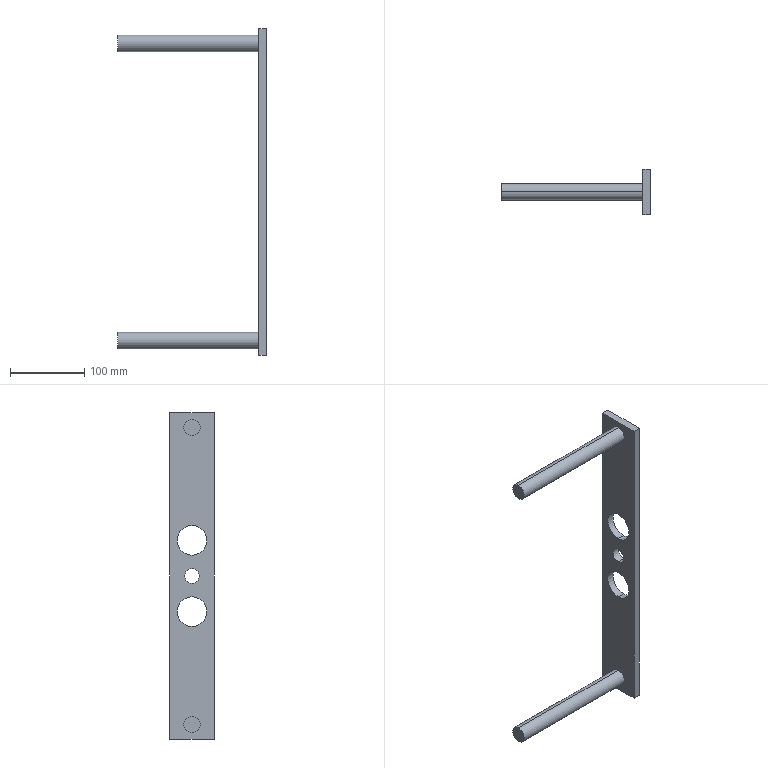Part | STEP file | 1 solid | 18 faces | box 200 x 60 x 440 mm | volume 380176 mm3 | cylinder 10 | plane 8 | commonest cylinder face diameters 22 x4 40 x4 20 x2
STEP:
#1=CARTESIAN_POINT('',(0.,0.,0.));
#2=DIRECTION('',(0.,0.,1.));
#3=DIRECTION('',(1.,0.,0.));
#4=AXIS2_PLACEMENT_3D('',#1,#2,#3);
#5=CARTESIAN_POINT('',(-10.,30.,-10.));
#6=VERTEX_POINT('',#5);
#7=CARTESIAN_POINT('',(0.,30.,-10.));
#8=VERTEX_POINT('',#7);
#9=CARTESIAN_POINT('',(13.,30.,-10.));
#10=DIRECTION('',(1.,0.,0.));
#11=VECTOR('',#10,1.);
#12=LINE('',#9,#11);
#13=CARTESIAN_POINT('',(13.,30.,0.));
#14=DIRECTION('',(1.,0.,0.));
#15=DIRECTION('',(0.,0.,-1.));
#16=AXIS2_PLACEMENT_3D('',#13,#14,#15);
#17=CYLINDRICAL_SURFACE('',#16,10.);
#18=CARTESIAN_POINT('',(6.283,0.));
#19=DIRECTION('',(0.,1.));
#20=VECTOR('',#19,1.);
#21=LINE('',#18,#20);
#22=(GEOMETRIC_REPRESENTATION_CONTEXT(2)PARAMETRIC_REPRESENTATION_CONTEXT()REPRESENTATION_CONTEXT('',''));
#23=DEFINITIONAL_REPRESENTATION('',(#21),#22);
#24=PCURVE('',#17,#23);
#25=CARTESIAN_POINT('',(13.,30.,0.));
#26=DIRECTION('',(1.,0.,0.));
#27=DIRECTION('',(0.,0.,-1.));
#28=AXIS2_PLACEMENT_3D('',#25,#26,#27);
#29=CYLINDRICAL_SURFACE('',#28,10.);
#30=CARTESIAN_POINT('',(0.,0.));
#31=DIRECTION('',(0.,1.));
#32=VECTOR('',#31,1.);
#33=LINE('',#30,#32);
#34=(GEOMETRIC_REPRESENTATION_CONTEXT(2)PARAMETRIC_REPRESENTATION_CONTEXT()REPRESENTATION_CONTEXT('',''));
#35=DEFINITIONAL_REPRESENTATION('',(#33),#34);
#36=PCURVE('',#29,#35);
#37=SURFACE_CURVE('',#12,(#24,#36),.PCURVE_S1.);
#38=EDGE_CURVE('',#6,#8,#37,.T.);
#39=ORIENTED_EDGE('',*,*,#38,.T.);
#40=CARTESIAN_POINT('',(0.,30.,10.));
#41=VERTEX_POINT('',#40);
#42=CARTESIAN_POINT('',(0.,30.,0.));
#43=DIRECTION('',(-1.,0.,0.));
#44=DIRECTION('',(0.,0.,-1.));
#45=AXIS2_PLACEMENT_3D('',#42,#43,#44);
#46=CIRCLE('',#45,10.);
#47=CARTESIAN_POINT('',(6.283,-13.));
#48=DIRECTION('',(-1.,0.));
#49=VECTOR('',#48,1.);
#50=LINE('',#47,#49);
#51=(GEOMETRIC_REPRESENTATION_CONTEXT(2)PARAMETRIC_REPRESENTATION_CONTEXT()REPRESENTATION_CONTEXT('',''));
#52=DEFINITIONAL_REPRESENTATION('',(#50),#51);
#53=PCURVE('',#17,#52);
#54=CARTESIAN_POINT('',(0.,60.,220.));
#55=DIRECTION('',(1.,0.,0.));
#56=DIRECTION('',(0.,1.,0.));
#57=AXIS2_PLACEMENT_3D('',#54,#55,#56);
#58=PLANE('',#57);
#59=CARTESIAN_POINT('',(-30.,-230.));
#60=CARTESIAN_POINT('',(-47.321,-230.));
#61=CARTESIAN_POINT('',(-38.66,-215.));
#62=CARTESIAN_POINT('',(-30.,-200.));
#63=CARTESIAN_POINT('',(-21.34,-215.));
#64=CARTESIAN_POINT('',(-12.679,-230.));
#65=CARTESIAN_POINT('',(-30.,-230.));
#66=(BOUNDED_CURVE()B_SPLINE_CURVE(2,(#59,#60,#61,#62,#63,#64,#65),.UNSPECIFIED.,.T.,.F.)B_SPLINE_CURVE_WITH_KNOTS((1,2,2,2,2,1),(-2.094,0.,2.094,4.189,6.283,8.378),.UNSPECIFIED.)CURVE()GEOMETRIC_REPRESENTATION_ITEM()RATIONAL_B_SPLINE_CURVE((1.,0.5,1.,0.5,1.,0.5,1.))REPRESENTATION_ITEM(''));
#67=(GEOMETRIC_REPRESENTATION_CONTEXT(2)PARAMETRIC_REPRESENTATION_CONTEXT()REPRESENTATION_CONTEXT('',''));
#68=DEFINITIONAL_REPRESENTATION('',(#66),#67);
#69=PCURVE('',#58,#68);
#70=SURFACE_CURVE('',#46,(#53,#69),.PCURVE_S1.);
#71=EDGE_CURVE('',#8,#41,#70,.T.);
#72=ORIENTED_EDGE('',*,*,#71,.T.);
#73=CARTESIAN_POINT('',(-10.,30.,10.));
#74=VERTEX_POINT('',#73);
#75=CARTESIAN_POINT('',(13.,30.,10.));
#76=DIRECTION('',(1.,0.,0.));
#77=VECTOR('',#76,1.);
#78=LINE('',#75,#77);
#79=CARTESIAN_POINT('',(3.142,0.));
#80=DIRECTION('',(0.,1.));
#81=VECTOR('',#80,1.);
#82=LINE('',#79,#81);
#83=(GEOMETRIC_REPRESENTATION_CONTEXT(2)PARAMETRIC_REPRESENTATION_CONTEXT()REPRESENTATION_CONTEXT('',''));
#84=DEFINITIONAL_REPRESENTATION('',(#82),#83);
#85=PCURVE('',#17,#84);
#86=CARTESIAN_POINT('',(3.142,0.));
#87=DIRECTION('',(0.,1.));
#88=VECTOR('',#87,1.);
#89=LINE('',#86,#88);
#90=(GEOMETRIC_REPRESENTATION_CONTEXT(2)PARAMETRIC_REPRESENTATION_CONTEXT()REPRESENTATION_CONTEXT('',''));
#91=DEFINITIONAL_REPRESENTATION('',(#89),#90);
#92=PCURVE('',#29,#91);
#93=SURFACE_CURVE('',#78,(#85,#92),.PCURVE_S1.);
#94=EDGE_CURVE('',#74,#41,#93,.T.);
#95=ORIENTED_EDGE('',*,*,#94,.F.);
#96=CARTESIAN_POINT('',(-10.,30.,0.));
#97=DIRECTION('',(1.,0.,0.));
#98=DIRECTION('',(0.,0.,-1.));
#99=AXIS2_PLACEMENT_3D('',#96,#97,#98);
#100=CIRCLE('',#99,10.);
#101=CARTESIAN_POINT('',(0.,-23.));
#102=DIRECTION('',(1.,0.));
#103=VECTOR('',#102,1.);
#104=LINE('',#101,#103);
#105=(GEOMETRIC_REPRESENTATION_CONTEXT(2)PARAMETRIC_REPRESENTATION_CONTEXT()REPRESENTATION_CONTEXT('',''));
#106=DEFINITIONAL_REPRESENTATION('',(#104),#105);
#107=PCURVE('',#17,#106);
#108=CARTESIAN_POINT('',(-10.,60.,220.));
#109=DIRECTION('',(1.,0.,0.));
#110=DIRECTION('',(0.,1.,0.));
#111=AXIS2_PLACEMENT_3D('',#108,#109,#110);
#112=PLANE('',#111);
#113=CARTESIAN_POINT('',(-30.,-220.));
#114=DIRECTION('',(0.,-1.));
#115=AXIS2_PLACEMENT_2D('',#113,#114);
#116=CIRCLE('',#115,10.);
#117=(GEOMETRIC_REPRESENTATION_CONTEXT(2)PARAMETRIC_REPRESENTATION_CONTEXT()REPRESENTATION_CONTEXT('',''));
#118=DEFINITIONAL_REPRESENTATION('',(#116),#117);
#119=PCURVE('',#112,#118);
#120=SURFACE_CURVE('',#100,(#107,#119),.PCURVE_S1.);
#121=EDGE_CURVE('',#74,#6,#120,.T.);
#122=ORIENTED_EDGE('',*,*,#121,.T.);
#123=EDGE_LOOP('',(#39,#72,#95,#122));
#124=FACE_BOUND('',#123,.F.);
#125=ADVANCED_FACE('',(#124),#17,.F.);
#126=CARTESIAN_POINT('',(-10.,30.,28.));
#127=VERTEX_POINT('',#126);
#128=CARTESIAN_POINT('',(0.,30.,28.));
#129=VERTEX_POINT('',#128);
#130=CARTESIAN_POINT('',(13.,30.,28.));
#131=DIRECTION('',(1.,0.,0.));
#132=VECTOR('',#131,1.);
#133=LINE('',#130,#132);
#134=CARTESIAN_POINT('',(13.,30.,48.));
#135=DIRECTION('',(1.,0.,0.));
#136=DIRECTION('',(0.,0.,-1.));
#137=AXIS2_PLACEMENT_3D('',#134,#135,#136);
#138=CYLINDRICAL_SURFACE('',#137,20.);
#139=CARTESIAN_POINT('',(6.283,0.));
#140=DIRECTION('',(0.,1.));
#141=VECTOR('',#140,1.);
#142=LINE('',#139,#141);
#143=(GEOMETRIC_REPRESENTATION_CONTEXT(2)PARAMETRIC_REPRESENTATION_CONTEXT()REPRESENTATION_CONTEXT('',''));
#144=DEFINITIONAL_REPRESENTATION('',(#142),#143);
#145=PCURVE('',#138,#144);
#146=CARTESIAN_POINT('',(13.,30.,48.));
#147=DIRECTION('',(1.,0.,0.));
#148=DIRECTION('',(0.,0.,-1.));
#149=AXIS2_PLACEMENT_3D('',#146,#147,#148);
#150=CYLINDRICAL_SURFACE('',#149,20.);
#151=CARTESIAN_POINT('',(0.,0.));
#152=DIRECTION('',(0.,1.));
#153=VECTOR('',#152,1.);
#154=LINE('',#151,#153);
#155=(GEOMETRIC_REPRESENTATION_CONTEXT(2)PARAMETRIC_REPRESENTATION_CONTEXT()REPRESENTATION_CONTEXT('',''));
#156=DEFINITIONAL_REPRESENTATION('',(#154),#155);
#157=PCURVE('',#150,#156);
#158=SURFACE_CURVE('',#133,(#145,#157),.PCURVE_S1.);
#159=EDGE_CURVE('',#127,#129,#158,.T.);
#160=ORIENTED_EDGE('',*,*,#159,.T.);
#161=CARTESIAN_POINT('',(0.,30.,68.));
#162=VERTEX_POINT('',#161);
#163=CARTESIAN_POINT('',(0.,30.,48.));
#164=DIRECTION('',(-1.,0.,0.));
#165=DIRECTION('',(0.,0.,-1.));
#166=AXIS2_PLACEMENT_3D('',#163,#164,#165);
#167=CIRCLE('',#166,20.);
#168=CARTESIAN_POINT('',(6.283,-13.));
#169=DIRECTION('',(-1.,0.));
#170=VECTOR('',#169,1.);
#171=LINE('',#168,#170);
#172=(GEOMETRIC_REPRESENTATION_CONTEXT(2)PARAMETRIC_REPRESENTATION_CONTEXT()REPRESENTATION_CONTEXT('',''));
#173=DEFINITIONAL_REPRESENTATION('',(#171),#172);
#174=PCURVE('',#138,#173);
#175=CARTESIAN_POINT('',(-30.,-192.));
#176=CARTESIAN_POINT('',(-64.641,-192.));
#177=CARTESIAN_POINT('',(-47.321,-162.));
#178=CARTESIAN_POINT('',(-30.,-132.));
#179=CARTESIAN_POINT('',(-12.679,-162.));
#180=CARTESIAN_POINT('',(4.641,-192.));
#181=CARTESIAN_POINT('',(-30.,-192.));
#182=(BOUNDED_CURVE()B_SPLINE_CURVE(2,(#175,#176,#177,#178,#179,#180,#181),.UNSPECIFIED.,.T.,.F.)B_SPLINE_CURVE_WITH_KNOTS((1,2,2,2,2,1),(-2.094,0.,2.094,4.189,6.283,8.378),.UNSPECIFIED.)CURVE()GEOMETRIC_REPRESENTATION_ITEM()RATIONAL_B_SPLINE_CURVE((1.,0.5,1.,0.5,1.,0.5,1.))REPRESENTATION_ITEM(''));
#183=(GEOMETRIC_REPRESENTATION_CONTEXT(2)PARAMETRIC_REPRESENTATION_CONTEXT()REPRESENTATION_CONTEXT('',''));
#184=DEFINITIONAL_REPRESENTATION('',(#182),#183);
#185=PCURVE('',#58,#184);
#186=SURFACE_CURVE('',#167,(#174,#185),.PCURVE_S1.);
#187=EDGE_CURVE('',#129,#162,#186,.T.);
#188=ORIENTED_EDGE('',*,*,#187,.T.);
#189=CARTESIAN_POINT('',(-10.,30.,68.));
#190=VERTEX_POINT('',#189);
#191=CARTESIAN_POINT('',(13.,30.,68.));
#192=DIRECTION('',(1.,0.,0.));
#193=VECTOR('',#192,1.);
#194=LINE('',#191,#193);
#195=CARTESIAN_POINT('',(3.142,0.));
#196=DIRECTION('',(0.,1.));
#197=VECTOR('',#196,1.);
#198=LINE('',#195,#197);
#199=(GEOMETRIC_REPRESENTATION_CONTEXT(2)PARAMETRIC_REPRESENTATION_CONTEXT()REPRESENTATION_CONTEXT('',''));
#200=DEFINITIONAL_REPRESENTATION('',(#198),#199);
#201=PCURVE('',#138,#200);
#202=CARTESIAN_POINT('',(3.142,0.));
#203=DIRECTION('',(0.,1.));
#204=VECTOR('',#203,1.);
#205=LINE('',#202,#204);
#206=(GEOMETRIC_REPRESENTATION_CONTEXT(2)PARAMETRIC_REPRESENTATION_CONTEXT()REPRESENTATION_CONTEXT('',''));
#207=DEFINITIONAL_REPRESENTATION('',(#205),#206);
#208=PCURVE('',#150,#207);
#209=SURFACE_CURVE('',#194,(#201,#208),.PCURVE_S1.);
#210=EDGE_CURVE('',#190,#162,#209,.T.);
#211=ORIENTED_EDGE('',*,*,#210,.F.);
#212=CARTESIAN_POINT('',(-10.,30.,48.));
#213=DIRECTION('',(1.,0.,0.));
#214=DIRECTION('',(0.,0.,-1.));
#215=AXIS2_PLACEMENT_3D('',#212,#213,#214);
#216=CIRCLE('',#215,20.);
#217=CARTESIAN_POINT('',(0.,-23.));
#218=DIRECTION('',(1.,0.));
#219=VECTOR('',#218,1.);
#220=LINE('',#217,#219);
#221=(GEOMETRIC_REPRESENTATION_CONTEXT(2)PARAMETRIC_REPRESENTATION_CONTEXT()REPRESENTATION_CONTEXT('',''));
#222=DEFINITIONAL_REPRESENTATION('',(#220),#221);
#223=PCURVE('',#138,#222);
#224=CARTESIAN_POINT('',(-30.,-172.));
#225=DIRECTION('',(0.,-1.));
#226=AXIS2_PLACEMENT_2D('',#224,#225);
#227=CIRCLE('',#226,20.);
#228=(GEOMETRIC_REPRESENTATION_CONTEXT(2)PARAMETRIC_REPRESENTATION_CONTEXT()REPRESENTATION_CONTEXT('',''));
#229=DEFINITIONAL_REPRESENTATION('',(#227),#228);
#230=PCURVE('',#112,#229);
#231=SURFACE_CURVE('',#216,(#223,#230),.PCURVE_S1.);
#232=EDGE_CURVE('',#190,#127,#231,.T.);
#233=ORIENTED_EDGE('',*,*,#232,.T.);
#234=EDGE_LOOP('',(#160,#188,#211,#233));
#235=FACE_BOUND('',#234,.F.);
#236=ADVANCED_FACE('',(#235),#138,.F.);
#237=CARTESIAN_POINT('',(-10.,30.,-68.));
#238=VERTEX_POINT('',#237);
#239=CARTESIAN_POINT('',(0.,30.,-68.));
#240=VERTEX_POINT('',#239);
#241=CARTESIAN_POINT('',(13.,30.,-68.));
#242=DIRECTION('',(1.,0.,0.));
#243=VECTOR('',#242,1.);
#244=LINE('',#241,#243);
#245=CARTESIAN_POINT('',(13.,30.,-48.));
#246=DIRECTION('',(1.,0.,0.));
#247=DIRECTION('',(0.,0.,-1.));
#248=AXIS2_PLACEMENT_3D('',#245,#246,#247);
#249=CYLINDRICAL_SURFACE('',#248,20.);
#250=CARTESIAN_POINT('',(6.283,0.));
#251=DIRECTION('',(0.,1.));
#252=VECTOR('',#251,1.);
#253=LINE('',#250,#252);
#254=(GEOMETRIC_REPRESENTATION_CONTEXT(2)PARAMETRIC_REPRESENTATION_CONTEXT()REPRESENTATION_CONTEXT('',''));
#255=DEFINITIONAL_REPRESENTATION('',(#253),#254);
#256=PCURVE('',#249,#255);
#257=CARTESIAN_POINT('',(13.,30.,-48.));
#258=DIRECTION('',(1.,0.,0.));
#259=DIRECTION('',(0.,0.,-1.));
#260=AXIS2_PLACEMENT_3D('',#257,#258,#259);
#261=CYLINDRICAL_SURFACE('',#260,20.);
#262=CARTESIAN_POINT('',(0.,0.));
#263=DIRECTION('',(0.,1.));
#264=VECTOR('',#263,1.);
#265=LINE('',#262,#264);
#266=(GEOMETRIC_REPRESENTATION_CONTEXT(2)PARAMETRIC_REPRESENTATION_CONTEXT()REPRESENTATION_CONTEXT('',''));
#267=DEFINITIONAL_REPRESENTATION('',(#265),#266);
#268=PCURVE('',#261,#267);
#269=SURFACE_CURVE('',#244,(#256,#268),.PCURVE_S1.);
#270=EDGE_CURVE('',#238,#240,#269,.T.);
#271=ORIENTED_EDGE('',*,*,#270,.T.);
#272=CARTESIAN_POINT('',(0.,30.,-28.));
#273=VERTEX_POINT('',#272);
#274=CARTESIAN_POINT('',(0.,30.,-48.));
#275=DIRECTION('',(-1.,0.,0.));
#276=DIRECTION('',(0.,0.,-1.));
#277=AXIS2_PLACEMENT_3D('',#274,#275,#276);
#278=CIRCLE('',#277,20.);
#279=CARTESIAN_POINT('',(6.283,-13.));
#280=DIRECTION('',(-1.,0.));
#281=VECTOR('',#280,1.);
#282=LINE('',#279,#281);
#283=(GEOMETRIC_REPRESENTATION_CONTEXT(2)PARAMETRIC_REPRESENTATION_CONTEXT()REPRESENTATION_CONTEXT('',''));
#284=DEFINITIONAL_REPRESENTATION('',(#282),#283);
#285=PCURVE('',#249,#284);
#286=CARTESIAN_POINT('',(-30.,-288.));
#287=CARTESIAN_POINT('',(-64.641,-288.));
#288=CARTESIAN_POINT('',(-47.321,-258.));
#289=CARTESIAN_POINT('',(-30.,-228.));
#290=CARTESIAN_POINT('',(-12.679,-258.));
#291=CARTESIAN_POINT('',(4.641,-288.));
#292=CARTESIAN_POINT('',(-30.,-288.));
#293=(BOUNDED_CURVE()B_SPLINE_CURVE(2,(#286,#287,#288,#289,#290,#291,#292),.UNSPECIFIED.,.T.,.F.)B_SPLINE_CURVE_WITH_KNOTS((1,2,2,2,2,1),(-2.094,0.,2.094,4.189,6.283,8.378),.UNSPECIFIED.)CURVE()GEOMETRIC_REPRESENTATION_ITEM()RATIONAL_B_SPLINE_CURVE((1.,0.5,1.,0.5,1.,0.5,1.))REPRESENTATION_ITEM(''));
#294=(GEOMETRIC_REPRESENTATION_CONTEXT(2)PARAMETRIC_REPRESENTATION_CONTEXT()REPRESENTATION_CONTEXT('',''));
#295=DEFINITIONAL_REPRESENTATION('',(#293),#294);
#296=PCURVE('',#58,#295);
#297=SURFACE_CURVE('',#278,(#285,#296),.PCURVE_S1.);
#298=EDGE_CURVE('',#240,#273,#297,.T.);
#299=ORIENTED_EDGE('',*,*,#298,.T.);
#300=CARTESIAN_POINT('',(-10.,30.,-28.));
#301=VERTEX_POINT('',#300);
#302=CARTESIAN_POINT('',(13.,30.,-28.));
#303=DIRECTION('',(1.,0.,0.));
#304=VECTOR('',#303,1.);
#305=LINE('',#302,#304);
#306=CARTESIAN_POINT('',(3.142,0.));
#307=DIRECTION('',(0.,1.));
#308=VECTOR('',#307,1.);
#309=LINE('',#306,#308);
#310=(GEOMETRIC_REPRESENTATION_CONTEXT(2)PARAMETRIC_REPRESENTATION_CONTEXT()REPRESENTATION_CONTEXT('',''));
#311=DEFINITIONAL_REPRESENTATION('',(#309),#310);
#312=PCURVE('',#249,#311);
#313=CARTESIAN_POINT('',(3.142,0.));
#314=DIRECTION('',(0.,1.));
#315=VECTOR('',#314,1.);
#316=LINE('',#313,#315);
#317=(GEOMETRIC_REPRESENTATION_CONTEXT(2)PARAMETRIC_REPRESENTATION_CONTEXT()REPRESENTATION_CONTEXT('',''));
#318=DEFINITIONAL_REPRESENTATION('',(#316),#317);
#319=PCURVE('',#261,#318);
#320=SURFACE_CURVE('',#305,(#312,#319),.PCURVE_S1.);
#321=EDGE_CURVE('',#301,#273,#320,.T.);
#322=ORIENTED_EDGE('',*,*,#321,.F.);
#323=CARTESIAN_POINT('',(-10.,30.,-48.));
#324=DIRECTION('',(1.,0.,0.));
#325=DIRECTION('',(0.,0.,-1.));
#326=AXIS2_PLACEMENT_3D('',#323,#324,#325);
#327=CIRCLE('',#326,20.);
#328=CARTESIAN_POINT('',(0.,-23.));
#329=DIRECTION('',(1.,0.));
#330=VECTOR('',#329,1.);
#331=LINE('',#328,#330);
#332=(GEOMETRIC_REPRESENTATION_CONTEXT(2)PARAMETRIC_REPRESENTATION_CONTEXT()REPRESENTATION_CONTEXT('',''));
#333=DEFINITIONAL_REPRESENTATION('',(#331),#332);
#334=PCURVE('',#249,#333);
#335=CARTESIAN_POINT('',(-30.,-268.));
#336=DIRECTION('',(0.,-1.));
#337=AXIS2_PLACEMENT_2D('',#335,#336);
#338=CIRCLE('',#337,20.);
#339=(GEOMETRIC_REPRESENTATION_CONTEXT(2)PARAMETRIC_REPRESENTATION_CONTEXT()REPRESENTATION_CONTEXT('',''));
#340=DEFINITIONAL_REPRESENTATION('',(#338),#339);
#341=PCURVE('',#112,#340);
#342=SURFACE_CURVE('',#327,(#334,#341),.PCURVE_S1.);
#343=EDGE_CURVE('',#301,#238,#342,.T.);
#344=ORIENTED_EDGE('',*,*,#343,.T.);
#345=EDGE_LOOP('',(#271,#299,#322,#344));
#346=FACE_BOUND('',#345,.F.);
#347=ADVANCED_FACE('',(#346),#249,.F.);
#348=CARTESIAN_POINT('',(-10.,30.,211.));
#349=VERTEX_POINT('',#348);
#350=CARTESIAN_POINT('',(-10.,30.,189.));
#351=VERTEX_POINT('',#350);
#352=CARTESIAN_POINT('',(-10.,30.,200.));
#353=DIRECTION('',(-1.,0.,0.));
#354=DIRECTION('',(0.,0.,1.));
#355=AXIS2_PLACEMENT_3D('',#352,#353,#354);
#356=CIRCLE('',#355,11.);
#357=CARTESIAN_POINT('',(-200.,30.,200.));
#358=DIRECTION('',(-1.,0.,0.));
#359=DIRECTION('',(0.,0.,1.));
#360=AXIS2_PLACEMENT_3D('',#357,#358,#359);
#361=CYLINDRICAL_SURFACE('',#360,11.);
#362=CARTESIAN_POINT('',(0.,-190.));
#363=DIRECTION('',(1.,0.));
#364=VECTOR('',#363,1.);
#365=LINE('',#362,#364);
#366=(GEOMETRIC_REPRESENTATION_CONTEXT(2)PARAMETRIC_REPRESENTATION_CONTEXT()REPRESENTATION_CONTEXT('',''));
#367=DEFINITIONAL_REPRESENTATION('',(#365),#366);
#368=PCURVE('',#361,#367);
#369=CARTESIAN_POINT('',(-30.,-9.));
#370=CARTESIAN_POINT('',(-10.947,-9.));
#371=CARTESIAN_POINT('',(-20.474,-25.5));
#372=CARTESIAN_POINT('',(-30.,-42.));
#373=CARTESIAN_POINT('',(-39.526,-25.5));
#374=CARTESIAN_POINT('',(-49.053,-9.));
#375=CARTESIAN_POINT('',(-30.,-9.));
#376=(BOUNDED_CURVE()B_SPLINE_CURVE(2,(#369,#370,#371,#372,#373,#374,#375),.UNSPECIFIED.,.T.,.F.)B_SPLINE_CURVE_WITH_KNOTS((1,2,2,2,2,1),(-2.094,0.,2.094,4.189,6.283,8.378),.UNSPECIFIED.)CURVE()GEOMETRIC_REPRESENTATION_ITEM()RATIONAL_B_SPLINE_CURVE((1.,0.5,1.,0.5,1.,0.5,1.))REPRESENTATION_ITEM(''));
#377=(GEOMETRIC_REPRESENTATION_CONTEXT(2)PARAMETRIC_REPRESENTATION_CONTEXT()REPRESENTATION_CONTEXT('',''));
#378=DEFINITIONAL_REPRESENTATION('',(#376),#377);
#379=PCURVE('',#112,#378);
#380=SURFACE_CURVE('',#356,(#368,#379),.PCURVE_S1.);
#381=EDGE_CURVE('',#349,#351,#380,.T.);
#382=ORIENTED_EDGE('',*,*,#381,.T.);
#383=CARTESIAN_POINT('',(-200.,30.,189.));
#384=VERTEX_POINT('',#383);
#385=CARTESIAN_POINT('',(-200.,30.,189.));
#386=DIRECTION('',(-1.,0.,0.));
#387=VECTOR('',#386,1.);
#388=LINE('',#385,#387);
#389=CARTESIAN_POINT('',(3.142,0.));
#390=DIRECTION('',(0.,1.));
#391=VECTOR('',#390,1.);
#392=LINE('',#389,#391);
#393=(GEOMETRIC_REPRESENTATION_CONTEXT(2)PARAMETRIC_REPRESENTATION_CONTEXT()REPRESENTATION_CONTEXT('',''));
#394=DEFINITIONAL_REPRESENTATION('',(#392),#393);
#395=PCURVE('',#361,#394);
#396=CARTESIAN_POINT('',(-200.,30.,200.));
#397=DIRECTION('',(-1.,0.,0.));
#398=DIRECTION('',(0.,0.,1.));
#399=AXIS2_PLACEMENT_3D('',#396,#397,#398);
#400=CYLINDRICAL_SURFACE('',#399,11.);
#401=CARTESIAN_POINT('',(3.142,0.));
#402=DIRECTION('',(0.,1.));
#403=VECTOR('',#402,1.);
#404=LINE('',#401,#403);
#405=(GEOMETRIC_REPRESENTATION_CONTEXT(2)PARAMETRIC_REPRESENTATION_CONTEXT()REPRESENTATION_CONTEXT('',''));
#406=DEFINITIONAL_REPRESENTATION('',(#404),#405);
#407=PCURVE('',#400,#406);
#408=SURFACE_CURVE('',#388,(#395,#407),.PCURVE_S1.);
#409=EDGE_CURVE('',#351,#384,#408,.T.);
#410=ORIENTED_EDGE('',*,*,#409,.T.);
#411=CARTESIAN_POINT('',(-200.,30.,211.));
#412=VERTEX_POINT('',#411);
#413=CARTESIAN_POINT('',(-200.,30.,200.));
#414=DIRECTION('',(1.,0.,0.));
#415=DIRECTION('',(0.,0.,1.));
#416=AXIS2_PLACEMENT_3D('',#413,#414,#415);
#417=CIRCLE('',#416,11.);
#418=CARTESIAN_POINT('',(6.283,0.));
#419=DIRECTION('',(-1.,0.));
#420=VECTOR('',#419,1.);
#421=LINE('',#418,#420);
#422=(GEOMETRIC_REPRESENTATION_CONTEXT(2)PARAMETRIC_REPRESENTATION_CONTEXT()REPRESENTATION_CONTEXT('',''));
#423=DEFINITIONAL_REPRESENTATION('',(#421),#422);
#424=PCURVE('',#361,#423);
#425=CARTESIAN_POINT('',(-200.,30.,200.));
#426=DIRECTION('',(1.,0.,0.));
#427=DIRECTION('',(0.,1.,0.));
#428=AXIS2_PLACEMENT_3D('',#425,#426,#427);
#429=PLANE('',#428);
#430=CARTESIAN_POINT('',(0.,0.));
#431=DIRECTION('',(0.,1.));
#432=AXIS2_PLACEMENT_2D('',#430,#431);
#433=CIRCLE('',#432,11.);
#434=(GEOMETRIC_REPRESENTATION_CONTEXT(2)PARAMETRIC_REPRESENTATION_CONTEXT()REPRESENTATION_CONTEXT('',''));
#435=DEFINITIONAL_REPRESENTATION('',(#433),#434);
#436=PCURVE('',#429,#435);
#437=SURFACE_CURVE('',#417,(#424,#436),.PCURVE_S1.);
#438=EDGE_CURVE('',#384,#412,#437,.T.);
#439=ORIENTED_EDGE('',*,*,#438,.T.);
#440=CARTESIAN_POINT('',(-200.,30.,211.));
#441=DIRECTION('',(-1.,0.,0.));
#442=VECTOR('',#441,1.);
#443=LINE('',#440,#442);
#444=CARTESIAN_POINT('',(0.,0.));
#445=DIRECTION('',(0.,1.));
#446=VECTOR('',#445,1.);
#447=LINE('',#444,#446);
#448=(GEOMETRIC_REPRESENTATION_CONTEXT(2)PARAMETRIC_REPRESENTATION_CONTEXT()REPRESENTATION_CONTEXT('',''));
#449=DEFINITIONAL_REPRESENTATION('',(#447),#448);
#450=PCURVE('',#361,#449);
#451=CARTESIAN_POINT('',(6.283,0.));
#452=DIRECTION('',(0.,1.));
#453=VECTOR('',#452,1.);
#454=LINE('',#451,#453);
#455=(GEOMETRIC_REPRESENTATION_CONTEXT(2)PARAMETRIC_REPRESENTATION_CONTEXT()REPRESENTATION_CONTEXT('',''));
#456=DEFINITIONAL_REPRESENTATION('',(#454),#455);
#457=PCURVE('',#400,#456);
#458=SURFACE_CURVE('',#443,(#450,#457),.PCURVE_S1.);
#459=EDGE_CURVE('',#349,#412,#458,.T.);
#460=ORIENTED_EDGE('',*,*,#459,.F.);
#461=EDGE_LOOP('',(#382,#410,#439,#460));
#462=FACE_BOUND('',#461,.T.);
#463=ADVANCED_FACE('',(#462),#361,.T.);
#464=CARTESIAN_POINT('',(-10.,30.,-189.));
#465=VERTEX_POINT('',#464);
#466=CARTESIAN_POINT('',(-10.,30.,-211.));
#467=VERTEX_POINT('',#466);
#468=CARTESIAN_POINT('',(-10.,30.,-200.));
#469=DIRECTION('',(-1.,0.,0.));
#470=DIRECTION('',(0.,0.,1.));
#471=AXIS2_PLACEMENT_3D('',#468,#469,#470);
#472=CIRCLE('',#471,11.);
#473=CARTESIAN_POINT('',(-200.,30.,-200.));
#474=DIRECTION('',(-1.,0.,0.));
#475=DIRECTION('',(0.,0.,1.));
#476=AXIS2_PLACEMENT_3D('',#473,#474,#475);
#477=CYLINDRICAL_SURFACE('',#476,11.);
#478=CARTESIAN_POINT('',(0.,-190.));
#479=DIRECTION('',(1.,0.));
#480=VECTOR('',#479,1.);
#481=LINE('',#478,#480);
#482=(GEOMETRIC_REPRESENTATION_CONTEXT(2)PARAMETRIC_REPRESENTATION_CONTEXT()REPRESENTATION_CONTEXT('',''));
#483=DEFINITIONAL_REPRESENTATION('',(#481),#482);
#484=PCURVE('',#477,#483);
#485=CARTESIAN_POINT('',(-30.,-409.));
#486=CARTESIAN_POINT('',(-10.947,-409.));
#487=CARTESIAN_POINT('',(-20.474,-425.5));
#488=CARTESIAN_POINT('',(-30.,-442.));
#489=CARTESIAN_POINT('',(-39.526,-425.5));
#490=CARTESIAN_POINT('',(-49.053,-409.));
#491=CARTESIAN_POINT('',(-30.,-409.));
#492=(BOUNDED_CURVE()B_SPLINE_CURVE(2,(#485,#486,#487,#488,#489,#490,#491),.UNSPECIFIED.,.T.,.F.)B_SPLINE_CURVE_WITH_KNOTS((1,2,2,2,2,1),(-2.094,0.,2.094,4.189,6.283,8.378),.UNSPECIFIED.)CURVE()GEOMETRIC_REPRESENTATION_ITEM()RATIONAL_B_SPLINE_CURVE((1.,0.5,1.,0.5,1.,0.5,1.))REPRESENTATION_ITEM(''));
#493=(GEOMETRIC_REPRESENTATION_CONTEXT(2)PARAMETRIC_REPRESENTATION_CONTEXT()REPRESENTATION_CONTEXT('',''));
#494=DEFINITIONAL_REPRESENTATION('',(#492),#493);
#495=PCURVE('',#112,#494);
#496=SURFACE_CURVE('',#472,(#484,#495),.PCURVE_S1.);
#497=EDGE_CURVE('',#465,#467,#496,.T.);
#498=ORIENTED_EDGE('',*,*,#497,.T.);
#499=CARTESIAN_POINT('',(-200.,30.,-211.));
#500=VERTEX_POINT('',#499);
#501=CARTESIAN_POINT('',(-200.,30.,-211.));
#502=DIRECTION('',(-1.,0.,0.));
#503=VECTOR('',#502,1.);
#504=LINE('',#501,#503);
#505=CARTESIAN_POINT('',(3.142,0.));
#506=DIRECTION('',(0.,1.));
#507=VECTOR('',#506,1.);
#508=LINE('',#505,#507);
#509=(GEOMETRIC_REPRESENTATION_CONTEXT(2)PARAMETRIC_REPRESENTATION_CONTEXT()REPRESENTATION_CONTEXT('',''));
#510=DEFINITIONAL_REPRESENTATION('',(#508),#509);
#511=PCURVE('',#477,#510);
#512=CARTESIAN_POINT('',(-200.,30.,-200.));
#513=DIRECTION('',(-1.,0.,0.));
#514=DIRECTION('',(0.,0.,1.));
#515=AXIS2_PLACEMENT_3D('',#512,#513,#514);
#516=CYLINDRICAL_SURFACE('',#515,11.);
#517=CARTESIAN_POINT('',(3.142,0.));
#518=DIRECTION('',(0.,1.));
#519=VECTOR('',#518,1.);
#520=LINE('',#517,#519);
#521=(GEOMETRIC_REPRESENTATION_CONTEXT(2)PARAMETRIC_REPRESENTATION_CONTEXT()REPRESENTATION_CONTEXT('',''));
#522=DEFINITIONAL_REPRESENTATION('',(#520),#521);
#523=PCURVE('',#516,#522);
#524=SURFACE_CURVE('',#504,(#511,#523),.PCURVE_S1.);
#525=EDGE_CURVE('',#467,#500,#524,.T.);
#526=ORIENTED_EDGE('',*,*,#525,.T.);
#527=CARTESIAN_POINT('',(-200.,30.,-189.));
#528=VERTEX_POINT('',#527);
#529=CARTESIAN_POINT('',(-200.,30.,-200.));
#530=DIRECTION('',(1.,0.,0.));
#531=DIRECTION('',(0.,0.,1.));
#532=AXIS2_PLACEMENT_3D('',#529,#530,#531);
#533=CIRCLE('',#532,11.);
#534=CARTESIAN_POINT('',(6.283,0.));
#535=DIRECTION('',(-1.,0.));
#536=VECTOR('',#535,1.);
#537=LINE('',#534,#536);
#538=(GEOMETRIC_REPRESENTATION_CONTEXT(2)PARAMETRIC_REPRESENTATION_CONTEXT()REPRESENTATION_CONTEXT('',''));
#539=DEFINITIONAL_REPRESENTATION('',(#537),#538);
#540=PCURVE('',#477,#539);
#541=CARTESIAN_POINT('',(-200.,30.,-200.));
#542=DIRECTION('',(-1.,0.,0.));
#543=DIRECTION('',(0.,-1.,0.));
#544=AXIS2_PLACEMENT_3D('',#541,#542,#543);
#545=PLANE('',#544);
#546=CARTESIAN_POINT('',(0.,11.));
#547=CARTESIAN_POINT('',(19.053,11.));
#548=CARTESIAN_POINT('',(9.526,-5.5));
#549=CARTESIAN_POINT('',(0.,-22.));
#550=CARTESIAN_POINT('',(-9.526,-5.5));
#551=CARTESIAN_POINT('',(-19.053,11.));
#552=CARTESIAN_POINT('',(0.,11.));
#553=(BOUNDED_CURVE()B_SPLINE_CURVE(2,(#546,#547,#548,#549,#550,#551,#552),.UNSPECIFIED.,.T.,.F.)B_SPLINE_CURVE_WITH_KNOTS((1,2,2,2,2,1),(-2.094,0.,2.094,4.189,6.283,8.378),.UNSPECIFIED.)CURVE()GEOMETRIC_REPRESENTATION_ITEM()RATIONAL_B_SPLINE_CURVE((1.,0.5,1.,0.5,1.,0.5,1.))REPRESENTATION_ITEM(''));
#554=(GEOMETRIC_REPRESENTATION_CONTEXT(2)PARAMETRIC_REPRESENTATION_CONTEXT()REPRESENTATION_CONTEXT('',''));
#555=DEFINITIONAL_REPRESENTATION('',(#553),#554);
#556=PCURVE('',#545,#555);
#557=SURFACE_CURVE('',#533,(#540,#556),.PCURVE_S1.);
#558=EDGE_CURVE('',#500,#528,#557,.T.);
#559=ORIENTED_EDGE('',*,*,#558,.T.);
#560=CARTESIAN_POINT('',(-200.,30.,-189.));
#561=DIRECTION('',(-1.,0.,0.));
#562=VECTOR('',#561,1.);
#563=LINE('',#560,#562);
#564=CARTESIAN_POINT('',(0.,0.));
#565=DIRECTION('',(0.,1.));
#566=VECTOR('',#565,1.);
#567=LINE('',#564,#566);
#568=(GEOMETRIC_REPRESENTATION_CONTEXT(2)PARAMETRIC_REPRESENTATION_CONTEXT()REPRESENTATION_CONTEXT('',''));
#569=DEFINITIONAL_REPRESENTATION('',(#567),#568);
#570=PCURVE('',#477,#569);
#571=CARTESIAN_POINT('',(6.283,0.));
#572=DIRECTION('',(0.,1.));
#573=VECTOR('',#572,1.);
#574=LINE('',#571,#573);
#575=(GEOMETRIC_REPRESENTATION_CONTEXT(2)PARAMETRIC_REPRESENTATION_CONTEXT()REPRESENTATION_CONTEXT('',''));
#576=DEFINITIONAL_REPRESENTATION('',(#574),#575);
#577=PCURVE('',#516,#576);
#578=SURFACE_CURVE('',#563,(#570,#577),.PCURVE_S1.);
#579=EDGE_CURVE('',#465,#528,#578,.T.);
#580=ORIENTED_EDGE('',*,*,#579,.F.);
#581=EDGE_LOOP('',(#498,#526,#559,#580));
#582=FACE_BOUND('',#581,.T.);
#583=ADVANCED_FACE('',(#582),#477,.T.);
#584=ORIENTED_EDGE('',*,*,#71,.T.);
#585=CARTESIAN_POINT('',(0.,30.,0.));
#586=DIRECTION('',(-1.,0.,0.));
#587=DIRECTION('',(0.,0.,-1.));
#588=AXIS2_PLACEMENT_3D('',#585,#586,#587);
#589=CIRCLE('',#588,10.);
#590=CARTESIAN_POINT('',(-30.,-230.));
#591=CARTESIAN_POINT('',(-47.321,-230.));
#592=CARTESIAN_POINT('',(-38.66,-215.));
#593=CARTESIAN_POINT('',(-30.,-200.));
#594=CARTESIAN_POINT('',(-21.34,-215.));
#595=CARTESIAN_POINT('',(-12.679,-230.));
#596=CARTESIAN_POINT('',(-30.,-230.));
#597=(BOUNDED_CURVE()B_SPLINE_CURVE(2,(#590,#591,#592,#593,#594,#595,#596),.UNSPECIFIED.,.T.,.F.)B_SPLINE_CURVE_WITH_KNOTS((1,2,2,2,2,1),(-2.094,0.,2.094,4.189,6.283,8.378),.UNSPECIFIED.)CURVE()GEOMETRIC_REPRESENTATION_ITEM()RATIONAL_B_SPLINE_CURVE((1.,0.5,1.,0.5,1.,0.5,1.))REPRESENTATION_ITEM(''));
#598=(GEOMETRIC_REPRESENTATION_CONTEXT(2)PARAMETRIC_REPRESENTATION_CONTEXT()REPRESENTATION_CONTEXT('',''));
#599=DEFINITIONAL_REPRESENTATION('',(#597),#598);
#600=PCURVE('',#58,#599);
#601=CARTESIAN_POINT('',(6.283,-13.));
#602=DIRECTION('',(-1.,0.));
#603=VECTOR('',#602,1.);
#604=LINE('',#601,#603);
#605=(GEOMETRIC_REPRESENTATION_CONTEXT(2)PARAMETRIC_REPRESENTATION_CONTEXT()REPRESENTATION_CONTEXT('',''));
#606=DEFINITIONAL_REPRESENTATION('',(#604),#605);
#607=PCURVE('',#29,#606);
#608=SURFACE_CURVE('',#589,(#600,#607),.PCURVE_S1.);
#609=EDGE_CURVE('',#41,#8,#608,.T.);
#610=ORIENTED_EDGE('',*,*,#609,.T.);
#611=EDGE_LOOP('',(#584,#610));
#612=FACE_BOUND('',#611,.T.);
#613=ORIENTED_EDGE('',*,*,#187,.T.);
#614=CARTESIAN_POINT('',(0.,30.,48.));
#615=DIRECTION('',(-1.,0.,0.));
#616=DIRECTION('',(0.,0.,-1.));
#617=AXIS2_PLACEMENT_3D('',#614,#615,#616);
#618=CIRCLE('',#617,20.);
#619=CARTESIAN_POINT('',(-30.,-192.));
#620=CARTESIAN_POINT('',(-64.641,-192.));
#621=CARTESIAN_POINT('',(-47.321,-162.));
#622=CARTESIAN_POINT('',(-30.,-132.));
#623=CARTESIAN_POINT('',(-12.679,-162.));
#624=CARTESIAN_POINT('',(4.641,-192.));
#625=CARTESIAN_POINT('',(-30.,-192.));
#626=(BOUNDED_CURVE()B_SPLINE_CURVE(2,(#619,#620,#621,#622,#623,#624,#625),.UNSPECIFIED.,.T.,.F.)B_SPLINE_CURVE_WITH_KNOTS((1,2,2,2,2,1),(-2.094,0.,2.094,4.189,6.283,8.378),.UNSPECIFIED.)CURVE()GEOMETRIC_REPRESENTATION_ITEM()RATIONAL_B_SPLINE_CURVE((1.,0.5,1.,0.5,1.,0.5,1.))REPRESENTATION_ITEM(''));
#627=(GEOMETRIC_REPRESENTATION_CONTEXT(2)PARAMETRIC_REPRESENTATION_CONTEXT()REPRESENTATION_CONTEXT('',''));
#628=DEFINITIONAL_REPRESENTATION('',(#626),#627);
#629=PCURVE('',#58,#628);
#630=CARTESIAN_POINT('',(6.283,-13.));
#631=DIRECTION('',(-1.,0.));
#632=VECTOR('',#631,1.);
#633=LINE('',#630,#632);
#634=(GEOMETRIC_REPRESENTATION_CONTEXT(2)PARAMETRIC_REPRESENTATION_CONTEXT()REPRESENTATION_CONTEXT('',''));
#635=DEFINITIONAL_REPRESENTATION('',(#633),#634);
#636=PCURVE('',#150,#635);
#637=SURFACE_CURVE('',#618,(#629,#636),.PCURVE_S1.);
#638=EDGE_CURVE('',#162,#129,#637,.T.);
#639=ORIENTED_EDGE('',*,*,#638,.T.);
#640=EDGE_LOOP('',(#613,#639));
#641=FACE_BOUND('',#640,.T.);
#642=ORIENTED_EDGE('',*,*,#298,.T.);
#643=CARTESIAN_POINT('',(0.,30.,-48.));
#644=DIRECTION('',(-1.,0.,0.));
#645=DIRECTION('',(0.,0.,-1.));
#646=AXIS2_PLACEMENT_3D('',#643,#644,#645);
#647=CIRCLE('',#646,20.);
#648=CARTESIAN_POINT('',(-30.,-288.));
#649=CARTESIAN_POINT('',(-64.641,-288.));
#650=CARTESIAN_POINT('',(-47.321,-258.));
#651=CARTESIAN_POINT('',(-30.,-228.));
#652=CARTESIAN_POINT('',(-12.679,-258.));
#653=CARTESIAN_POINT('',(4.641,-288.));
#654=CARTESIAN_POINT('',(-30.,-288.));
#655=(BOUNDED_CURVE()B_SPLINE_CURVE(2,(#648,#649,#650,#651,#652,#653,#654),.UNSPECIFIED.,.T.,.F.)B_SPLINE_CURVE_WITH_KNOTS((1,2,2,2,2,1),(-2.094,0.,2.094,4.189,6.283,8.378),.UNSPECIFIED.)CURVE()GEOMETRIC_REPRESENTATION_ITEM()RATIONAL_B_SPLINE_CURVE((1.,0.5,1.,0.5,1.,0.5,1.))REPRESENTATION_ITEM(''));
#656=(GEOMETRIC_REPRESENTATION_CONTEXT(2)PARAMETRIC_REPRESENTATION_CONTEXT()REPRESENTATION_CONTEXT('',''));
#657=DEFINITIONAL_REPRESENTATION('',(#655),#656);
#658=PCURVE('',#58,#657);
#659=CARTESIAN_POINT('',(6.283,-13.));
#660=DIRECTION('',(-1.,0.));
#661=VECTOR('',#660,1.);
#662=LINE('',#659,#661);
#663=(GEOMETRIC_REPRESENTATION_CONTEXT(2)PARAMETRIC_REPRESENTATION_CONTEXT()REPRESENTATION_CONTEXT('',''));
#664=DEFINITIONAL_REPRESENTATION('',(#662),#663);
#665=PCURVE('',#261,#664);
#666=SURFACE_CURVE('',#647,(#658,#665),.PCURVE_S1.);
#667=EDGE_CURVE('',#273,#240,#666,.T.);
#668=ORIENTED_EDGE('',*,*,#667,.T.);
#669=EDGE_LOOP('',(#642,#668));
#670=FACE_BOUND('',#669,.T.);
#671=CARTESIAN_POINT('',(0.,60.,220.));
#672=VERTEX_POINT('',#671);
#673=CARTESIAN_POINT('',(0.,0.,220.));
#674=VERTEX_POINT('',#673);
#675=CARTESIAN_POINT('',(0.,60.,220.));
#676=DIRECTION('',(0.,-1.,0.));
#677=VECTOR('',#676,1.);
#678=LINE('',#675,#677);
#679=CARTESIAN_POINT('',(0.,0.));
#680=DIRECTION('',(-1.,0.));
#681=VECTOR('',#680,1.);
#682=LINE('',#679,#681);
#683=(GEOMETRIC_REPRESENTATION_CONTEXT(2)PARAMETRIC_REPRESENTATION_CONTEXT()REPRESENTATION_CONTEXT('',''));
#684=DEFINITIONAL_REPRESENTATION('',(#682),#683);
#685=PCURVE('',#58,#684);
#686=CARTESIAN_POINT('',(0.,0.,220.));
#687=DIRECTION('',(0.,0.,-1.));
#688=DIRECTION('',(-1.,0.,0.));
#689=AXIS2_PLACEMENT_3D('',#686,#687,#688);
#690=PLANE('',#689);
#691=CARTESIAN_POINT('',(0.,60.));
#692=DIRECTION('',(0.,-1.));
#693=VECTOR('',#692,1.);
#694=LINE('',#691,#693);
#695=(GEOMETRIC_REPRESENTATION_CONTEXT(2)PARAMETRIC_REPRESENTATION_CONTEXT()REPRESENTATION_CONTEXT('',''));
#696=DEFINITIONAL_REPRESENTATION('',(#694),#695);
#697=PCURVE('',#690,#696);
#698=SURFACE_CURVE('',#678,(#685,#697),.PCURVE_S1.);
#699=EDGE_CURVE('',#672,#674,#698,.T.);
#700=ORIENTED_EDGE('',*,*,#699,.T.);
#701=CARTESIAN_POINT('',(0.,0.,-220.));
#702=VERTEX_POINT('',#701);
#703=CARTESIAN_POINT('',(0.,0.,220.));
#704=DIRECTION('',(0.,0.,-1.));
#705=VECTOR('',#704,1.);
#706=LINE('',#703,#705);
#707=CARTESIAN_POINT('',(-60.,0.));
#708=DIRECTION('',(0.,-1.));
#709=VECTOR('',#708,1.);
#710=LINE('',#707,#709);
#711=(GEOMETRIC_REPRESENTATION_CONTEXT(2)PARAMETRIC_REPRESENTATION_CONTEXT()REPRESENTATION_CONTEXT('',''));
#712=DEFINITIONAL_REPRESENTATION('',(#710),#711);
#713=PCURVE('',#58,#712);
#714=CARTESIAN_POINT('',(0.,0.,220.));
#715=DIRECTION('',(0.,-1.,0.));
#716=DIRECTION('',(0.,0.,-1.));
#717=AXIS2_PLACEMENT_3D('',#714,#715,#716);
#718=PLANE('',#717);
#719=CARTESIAN_POINT('',(0.,0.));
#720=DIRECTION('',(1.,0.));
#721=VECTOR('',#720,1.);
#722=LINE('',#719,#721);
#723=(GEOMETRIC_REPRESENTATION_CONTEXT(2)PARAMETRIC_REPRESENTATION_CONTEXT()REPRESENTATION_CONTEXT('',''));
#724=DEFINITIONAL_REPRESENTATION('',(#722),#723);
#725=PCURVE('',#718,#724);
#726=SURFACE_CURVE('',#706,(#713,#725),.PCURVE_S1.);
#727=EDGE_CURVE('',#674,#702,#726,.T.);
#728=ORIENTED_EDGE('',*,*,#727,.T.);
#729=CARTESIAN_POINT('',(0.,60.,-220.));
#730=VERTEX_POINT('',#729);
#731=CARTESIAN_POINT('',(0.,60.,-220.));
#732=DIRECTION('',(0.,1.,0.));
#733=VECTOR('',#732,1.);
#734=LINE('',#731,#733);
#735=CARTESIAN_POINT('',(0.,-440.));
#736=DIRECTION('',(1.,0.));
#737=VECTOR('',#736,1.);
#738=LINE('',#735,#737);
#739=(GEOMETRIC_REPRESENTATION_CONTEXT(2)PARAMETRIC_REPRESENTATION_CONTEXT()REPRESENTATION_CONTEXT('',''));
#740=DEFINITIONAL_REPRESENTATION('',(#738),#739);
#741=PCURVE('',#58,#740);
#742=CARTESIAN_POINT('',(0.,0.,-220.));
#743=DIRECTION('',(0.,0.,-1.));
#744=DIRECTION('',(-1.,0.,0.));
#745=AXIS2_PLACEMENT_3D('',#742,#743,#744);
#746=PLANE('',#745);
#747=CARTESIAN_POINT('',(0.,60.));
#748=DIRECTION('',(0.,1.));
#749=VECTOR('',#748,1.);
#750=LINE('',#747,#749);
#751=(GEOMETRIC_REPRESENTATION_CONTEXT(2)PARAMETRIC_REPRESENTATION_CONTEXT()REPRESENTATION_CONTEXT('',''));
#752=DEFINITIONAL_REPRESENTATION('',(#750),#751);
#753=PCURVE('',#746,#752);
#754=SURFACE_CURVE('',#734,(#741,#753),.PCURVE_S1.);
#755=EDGE_CURVE('',#702,#730,#754,.T.);
#756=ORIENTED_EDGE('',*,*,#755,.T.);
#757=CARTESIAN_POINT('',(0.,60.,220.));
#758=DIRECTION('',(0.,0.,1.));
#759=VECTOR('',#758,1.);
#760=LINE('',#757,#759);
#761=CARTESIAN_POINT('',(0.,0.));
#762=DIRECTION('',(0.,1.));
#763=VECTOR('',#762,1.);
#764=LINE('',#761,#763);
#765=(GEOMETRIC_REPRESENTATION_CONTEXT(2)PARAMETRIC_REPRESENTATION_CONTEXT()REPRESENTATION_CONTEXT('',''));
#766=DEFINITIONAL_REPRESENTATION('',(#764),#765);
#767=PCURVE('',#58,#766);
#768=CARTESIAN_POINT('',(-10.,60.,220.));
#769=DIRECTION('',(0.,1.,0.));
#770=DIRECTION('',(0.,0.,1.));
#771=AXIS2_PLACEMENT_3D('',#768,#769,#770);
#772=PLANE('',#771);
#773=CARTESIAN_POINT('',(0.,10.));
#774=DIRECTION('',(1.,0.));
#775=VECTOR('',#774,1.);
#776=LINE('',#773,#775);
#777=(GEOMETRIC_REPRESENTATION_CONTEXT(2)PARAMETRIC_REPRESENTATION_CONTEXT()REPRESENTATION_CONTEXT('',''));
#778=DEFINITIONAL_REPRESENTATION('',(#776),#777);
#779=PCURVE('',#772,#778);
#780=SURFACE_CURVE('',#760,(#767,#779),.PCURVE_S1.);
#781=EDGE_CURVE('',#730,#672,#780,.T.);
#782=ORIENTED_EDGE('',*,*,#781,.T.);
#783=EDGE_LOOP('',(#700,#728,#756,#782));
#784=FACE_BOUND('',#783,.T.);
#785=ADVANCED_FACE('',(#612,#641,#670,#784),#58,.T.);
#786=ORIENTED_EDGE('',*,*,#609,.T.);
#787=ORIENTED_EDGE('',*,*,#38,.F.);
#788=CARTESIAN_POINT('',(-10.,30.,0.));
#789=DIRECTION('',(1.,0.,0.));
#790=DIRECTION('',(0.,0.,-1.));
#791=AXIS2_PLACEMENT_3D('',#788,#789,#790);
#792=CIRCLE('',#791,10.);
#793=CARTESIAN_POINT('',(0.,-23.));
#794=DIRECTION('',(1.,0.));
#795=VECTOR('',#794,1.);
#796=LINE('',#793,#795);
#797=(GEOMETRIC_REPRESENTATION_CONTEXT(2)PARAMETRIC_REPRESENTATION_CONTEXT()REPRESENTATION_CONTEXT('',''));
#798=DEFINITIONAL_REPRESENTATION('',(#796),#797);
#799=PCURVE('',#29,#798);
#800=CARTESIAN_POINT('',(-30.,-220.));
#801=DIRECTION('',(0.,-1.));
#802=AXIS2_PLACEMENT_2D('',#800,#801);
#803=CIRCLE('',#802,10.);
#804=(GEOMETRIC_REPRESENTATION_CONTEXT(2)PARAMETRIC_REPRESENTATION_CONTEXT()REPRESENTATION_CONTEXT('',''));
#805=DEFINITIONAL_REPRESENTATION('',(#803),#804);
#806=PCURVE('',#112,#805);
#807=SURFACE_CURVE('',#792,(#799,#806),.PCURVE_S1.);
#808=EDGE_CURVE('',#6,#74,#807,.T.);
#809=ORIENTED_EDGE('',*,*,#808,.T.);
#810=ORIENTED_EDGE('',*,*,#94,.T.);
#811=EDGE_LOOP('',(#786,#787,#809,#810));
#812=FACE_BOUND('',#811,.F.);
#813=ADVANCED_FACE('',(#812),#29,.F.);
#814=ORIENTED_EDGE('',*,*,#638,.T.);
#815=ORIENTED_EDGE('',*,*,#159,.F.);
#816=CARTESIAN_POINT('',(-10.,30.,48.));
#817=DIRECTION('',(1.,0.,0.));
#818=DIRECTION('',(0.,0.,-1.));
#819=AXIS2_PLACEMENT_3D('',#816,#817,#818);
#820=CIRCLE('',#819,20.);
#821=CARTESIAN_POINT('',(0.,-23.));
#822=DIRECTION('',(1.,0.));
#823=VECTOR('',#822,1.);
#824=LINE('',#821,#823);
#825=(GEOMETRIC_REPRESENTATION_CONTEXT(2)PARAMETRIC_REPRESENTATION_CONTEXT()REPRESENTATION_CONTEXT('',''));
#826=DEFINITIONAL_REPRESENTATION('',(#824),#825);
#827=PCURVE('',#150,#826);
#828=CARTESIAN_POINT('',(-30.,-172.));
#829=DIRECTION('',(0.,-1.));
#830=AXIS2_PLACEMENT_2D('',#828,#829);
#831=CIRCLE('',#830,20.);
#832=(GEOMETRIC_REPRESENTATION_CONTEXT(2)PARAMETRIC_REPRESENTATION_CONTEXT()REPRESENTATION_CONTEXT('',''));
#833=DEFINITIONAL_REPRESENTATION('',(#831),#832);
#834=PCURVE('',#112,#833);
#835=SURFACE_CURVE('',#820,(#827,#834),.PCURVE_S1.);
#836=EDGE_CURVE('',#127,#190,#835,.T.);
#837=ORIENTED_EDGE('',*,*,#836,.T.);
#838=ORIENTED_EDGE('',*,*,#210,.T.);
#839=EDGE_LOOP('',(#814,#815,#837,#838));
#840=FACE_BOUND('',#839,.F.);
#841=ADVANCED_FACE('',(#840),#150,.F.);
#842=ORIENTED_EDGE('',*,*,#667,.T.);
#843=ORIENTED_EDGE('',*,*,#270,.F.);
#844=CARTESIAN_POINT('',(-10.,30.,-48.));
#845=DIRECTION('',(1.,0.,0.));
#846=DIRECTION('',(0.,0.,-1.));
#847=AXIS2_PLACEMENT_3D('',#844,#845,#846);
#848=CIRCLE('',#847,20.);
#849=CARTESIAN_POINT('',(0.,-23.));
#850=DIRECTION('',(1.,0.));
#851=VECTOR('',#850,1.);
#852=LINE('',#849,#851);
#853=(GEOMETRIC_REPRESENTATION_CONTEXT(2)PARAMETRIC_REPRESENTATION_CONTEXT()REPRESENTATION_CONTEXT('',''));
#854=DEFINITIONAL_REPRESENTATION('',(#852),#853);
#855=PCURVE('',#261,#854);
#856=CARTESIAN_POINT('',(-30.,-268.));
#857=DIRECTION('',(0.,-1.));
#858=AXIS2_PLACEMENT_2D('',#856,#857);
#859=CIRCLE('',#858,20.);
#860=(GEOMETRIC_REPRESENTATION_CONTEXT(2)PARAMETRIC_REPRESENTATION_CONTEXT()REPRESENTATION_CONTEXT('',''));
#861=DEFINITIONAL_REPRESENTATION('',(#859),#860);
#862=PCURVE('',#112,#861);
#863=SURFACE_CURVE('',#848,(#855,#862),.PCURVE_S1.);
#864=EDGE_CURVE('',#238,#301,#863,.T.);
#865=ORIENTED_EDGE('',*,*,#864,.T.);
#866=ORIENTED_EDGE('',*,*,#321,.T.);
#867=EDGE_LOOP('',(#842,#843,#865,#866));
#868=FACE_BOUND('',#867,.F.);
#869=ADVANCED_FACE('',(#868),#261,.F.);
#870=CARTESIAN_POINT('',(-10.,0.,220.));
#871=VERTEX_POINT('',#870);
#872=CARTESIAN_POINT('',(0.,0.,220.));
#873=DIRECTION('',(-1.,0.,0.));
#874=VECTOR('',#873,1.);
#875=LINE('',#872,#874);
#876=CARTESIAN_POINT('',(0.,0.));
#877=DIRECTION('',(0.,-1.));
#878=VECTOR('',#877,1.);
#879=LINE('',#876,#878);
#880=(GEOMETRIC_REPRESENTATION_CONTEXT(2)PARAMETRIC_REPRESENTATION_CONTEXT()REPRESENTATION_CONTEXT('',''));
#881=DEFINITIONAL_REPRESENTATION('',(#879),#880);
#882=PCURVE('',#718,#881);
#883=CARTESIAN_POINT('',(0.,0.));
#884=DIRECTION('',(1.,0.));
#885=VECTOR('',#884,1.);
#886=LINE('',#883,#885);
#887=(GEOMETRIC_REPRESENTATION_CONTEXT(2)PARAMETRIC_REPRESENTATION_CONTEXT()REPRESENTATION_CONTEXT('',''));
#888=DEFINITIONAL_REPRESENTATION('',(#886),#887);
#889=PCURVE('',#690,#888);
#890=SURFACE_CURVE('',#875,(#882,#889),.PCURVE_S1.);
#891=EDGE_CURVE('',#674,#871,#890,.T.);
#892=ORIENTED_EDGE('',*,*,#891,.T.);
#893=CARTESIAN_POINT('',(-10.,0.,-220.));
#894=VERTEX_POINT('',#893);
#895=CARTESIAN_POINT('',(-10.,0.,220.));
#896=DIRECTION('',(0.,0.,-1.));
#897=VECTOR('',#896,1.);
#898=LINE('',#895,#897);
#899=CARTESIAN_POINT('',(0.,-10.));
#900=DIRECTION('',(1.,0.));
#901=VECTOR('',#900,1.);
#902=LINE('',#899,#901);
#903=(GEOMETRIC_REPRESENTATION_CONTEXT(2)PARAMETRIC_REPRESENTATION_CONTEXT()REPRESENTATION_CONTEXT('',''));
#904=DEFINITIONAL_REPRESENTATION('',(#902),#903);
#905=PCURVE('',#718,#904);
#906=CARTESIAN_POINT('',(-60.,0.));
#907=DIRECTION('',(0.,-1.));
#908=VECTOR('',#907,1.);
#909=LINE('',#906,#908);
#910=(GEOMETRIC_REPRESENTATION_CONTEXT(2)PARAMETRIC_REPRESENTATION_CONTEXT()REPRESENTATION_CONTEXT('',''));
#911=DEFINITIONAL_REPRESENTATION('',(#909),#910);
#912=PCURVE('',#112,#911);
#913=SURFACE_CURVE('',#898,(#905,#912),.PCURVE_S1.);
#914=EDGE_CURVE('',#871,#894,#913,.T.);
#915=ORIENTED_EDGE('',*,*,#914,.T.);
#916=CARTESIAN_POINT('',(0.,0.,-220.));
#917=DIRECTION('',(1.,0.,0.));
#918=VECTOR('',#917,1.);
#919=LINE('',#916,#918);
#920=CARTESIAN_POINT('',(440.,0.));
#921=DIRECTION('',(0.,1.));
#922=VECTOR('',#921,1.);
#923=LINE('',#920,#922);
#924=(GEOMETRIC_REPRESENTATION_CONTEXT(2)PARAMETRIC_REPRESENTATION_CONTEXT()REPRESENTATION_CONTEXT('',''));
#925=DEFINITIONAL_REPRESENTATION('',(#923),#924);
#926=PCURVE('',#718,#925);
#927=CARTESIAN_POINT('',(0.,0.));
#928=DIRECTION('',(-1.,0.));
#929=VECTOR('',#928,1.);
#930=LINE('',#927,#929);
#931=(GEOMETRIC_REPRESENTATION_CONTEXT(2)PARAMETRIC_REPRESENTATION_CONTEXT()REPRESENTATION_CONTEXT('',''));
#932=DEFINITIONAL_REPRESENTATION('',(#930),#931);
#933=PCURVE('',#746,#932);
#934=SURFACE_CURVE('',#919,(#926,#933),.PCURVE_S1.);
#935=EDGE_CURVE('',#894,#702,#934,.T.);
#936=ORIENTED_EDGE('',*,*,#935,.T.);
#937=ORIENTED_EDGE('',*,*,#727,.F.);
#938=EDGE_LOOP('',(#892,#915,#936,#937));
#939=FACE_BOUND('',#938,.T.);
#940=ADVANCED_FACE('',(#939),#718,.T.);
#941=ORIENTED_EDGE('',*,*,#891,.F.);
#942=ORIENTED_EDGE('',*,*,#699,.F.);
#943=CARTESIAN_POINT('',(-10.,60.,220.));
#944=VERTEX_POINT('',#943);
#945=CARTESIAN_POINT('',(0.,60.,220.));
#946=DIRECTION('',(1.,0.,0.));
#947=VECTOR('',#946,1.);
#948=LINE('',#945,#947);
#949=CARTESIAN_POINT('',(0.,60.));
#950=DIRECTION('',(-1.,0.));
#951=VECTOR('',#950,1.);
#952=LINE('',#949,#951);
#953=(GEOMETRIC_REPRESENTATION_CONTEXT(2)PARAMETRIC_REPRESENTATION_CONTEXT()REPRESENTATION_CONTEXT('',''));
#954=DEFINITIONAL_REPRESENTATION('',(#952),#953);
#955=PCURVE('',#690,#954);
#956=CARTESIAN_POINT('',(0.,10.));
#957=DIRECTION('',(0.,1.));
#958=VECTOR('',#957,1.);
#959=LINE('',#956,#958);
#960=(GEOMETRIC_REPRESENTATION_CONTEXT(2)PARAMETRIC_REPRESENTATION_CONTEXT()REPRESENTATION_CONTEXT('',''));
#961=DEFINITIONAL_REPRESENTATION('',(#959),#960);
#962=PCURVE('',#772,#961);
#963=SURFACE_CURVE('',#948,(#955,#962),.PCURVE_S1.);
#964=EDGE_CURVE('',#944,#672,#963,.T.);
#965=ORIENTED_EDGE('',*,*,#964,.F.);
#966=CARTESIAN_POINT('',(-10.,0.,220.));
#967=DIRECTION('',(0.,1.,0.));
#968=VECTOR('',#967,1.);
#969=LINE('',#966,#968);
#970=CARTESIAN_POINT('',(10.,0.));
#971=DIRECTION('',(0.,1.));
#972=VECTOR('',#971,1.);
#973=LINE('',#970,#972);
#974=(GEOMETRIC_REPRESENTATION_CONTEXT(2)PARAMETRIC_REPRESENTATION_CONTEXT()REPRESENTATION_CONTEXT('',''));
#975=DEFINITIONAL_REPRESENTATION('',(#973),#974);
#976=PCURVE('',#690,#975);
#977=CARTESIAN_POINT('',(-60.,0.));
#978=DIRECTION('',(1.,0.));
#979=VECTOR('',#978,1.);
#980=LINE('',#977,#979);
#981=(GEOMETRIC_REPRESENTATION_CONTEXT(2)PARAMETRIC_REPRESENTATION_CONTEXT()REPRESENTATION_CONTEXT('',''));
#982=DEFINITIONAL_REPRESENTATION('',(#980),#981);
#983=PCURVE('',#112,#982);
#984=SURFACE_CURVE('',#969,(#976,#983),.PCURVE_S1.);
#985=EDGE_CURVE('',#871,#944,#984,.T.);
#986=ORIENTED_EDGE('',*,*,#985,.F.);
#987=EDGE_LOOP('',(#941,#942,#965,#986));
#988=FACE_BOUND('',#987,.T.);
#989=ADVANCED_FACE('',(#988),#690,.F.);
#990=ORIENTED_EDGE('',*,*,#964,.T.);
#991=ORIENTED_EDGE('',*,*,#781,.F.);
#992=CARTESIAN_POINT('',(-10.,60.,-220.));
#993=VERTEX_POINT('',#992);
#994=CARTESIAN_POINT('',(-10.,60.,-220.));
#995=DIRECTION('',(-1.,0.,0.));
#996=VECTOR('',#995,1.);
#997=LINE('',#994,#996);
#998=CARTESIAN_POINT('',(-440.,0.));
#999=DIRECTION('',(0.,-1.));
#1000=VECTOR('',#999,1.);
#1001=LINE('',#998,#1000);
#1002=(GEOMETRIC_REPRESENTATION_CONTEXT(2)PARAMETRIC_REPRESENTATION_CONTEXT()REPRESENTATION_CONTEXT('',''));
#1003=DEFINITIONAL_REPRESENTATION('',(#1001),#1002);
#1004=PCURVE('',#772,#1003);
#1005=CARTESIAN_POINT('',(10.,60.));
#1006=DIRECTION('',(1.,0.));
#1007=VECTOR('',#1006,1.);
#1008=LINE('',#1005,#1007);
#1009=(GEOMETRIC_REPRESENTATION_CONTEXT(2)PARAMETRIC_REPRESENTATION_CONTEXT()REPRESENTATION_CONTEXT('',''));
#1010=DEFINITIONAL_REPRESENTATION('',(#1008),#1009);
#1011=PCURVE('',#746,#1010);
#1012=SURFACE_CURVE('',#997,(#1004,#1011),.PCURVE_S1.);
#1013=EDGE_CURVE('',#730,#993,#1012,.T.);
#1014=ORIENTED_EDGE('',*,*,#1013,.T.);
#1015=CARTESIAN_POINT('',(-10.,60.,220.));
#1016=DIRECTION('',(0.,0.,1.));
#1017=VECTOR('',#1016,1.);
#1018=LINE('',#1015,#1017);
#1019=CARTESIAN_POINT('',(0.,0.));
#1020=DIRECTION('',(1.,0.));
#1021=VECTOR('',#1020,1.);
#1022=LINE('',#1019,#1021);
#1023=(GEOMETRIC_REPRESENTATION_CONTEXT(2)PARAMETRIC_REPRESENTATION_CONTEXT()REPRESENTATION_CONTEXT('',''));
#1024=DEFINITIONAL_REPRESENTATION('',(#1022),#1023);
#1025=PCURVE('',#772,#1024);
#1026=CARTESIAN_POINT('',(0.,0.));
#1027=DIRECTION('',(0.,1.));
#1028=VECTOR('',#1027,1.);
#1029=LINE('',#1026,#1028);
#1030=(GEOMETRIC_REPRESENTATION_CONTEXT(2)PARAMETRIC_REPRESENTATION_CONTEXT()REPRESENTATION_CONTEXT('',''));
#1031=DEFINITIONAL_REPRESENTATION('',(#1029),#1030);
#1032=PCURVE('',#112,#1031);
#1033=SURFACE_CURVE('',#1018,(#1025,#1032),.PCURVE_S1.);
#1034=EDGE_CURVE('',#993,#944,#1033,.T.);
#1035=ORIENTED_EDGE('',*,*,#1034,.T.);
#1036=EDGE_LOOP('',(#990,#991,#1014,#1035));
#1037=FACE_BOUND('',#1036,.T.);
#1038=ADVANCED_FACE('',(#1037),#772,.T.);
#1039=ORIENTED_EDGE('',*,*,#755,.F.);
#1040=ORIENTED_EDGE('',*,*,#935,.F.);
#1041=CARTESIAN_POINT('',(-10.,0.,-220.));
#1042=DIRECTION('',(0.,1.,0.));
#1043=VECTOR('',#1042,1.);
#1044=LINE('',#1041,#1043);
#1045=CARTESIAN_POINT('',(10.,0.));
#1046=DIRECTION('',(0.,1.));
#1047=VECTOR('',#1046,1.);
#1048=LINE('',#1045,#1047);
#1049=(GEOMETRIC_REPRESENTATION_CONTEXT(2)PARAMETRIC_REPRESENTATION_CONTEXT()REPRESENTATION_CONTEXT('',''));
#1050=DEFINITIONAL_REPRESENTATION('',(#1048),#1049);
#1051=PCURVE('',#746,#1050);
#1052=CARTESIAN_POINT('',(-60.,-440.));
#1053=DIRECTION('',(1.,0.));
#1054=VECTOR('',#1053,1.);
#1055=LINE('',#1052,#1054);
#1056=(GEOMETRIC_REPRESENTATION_CONTEXT(2)PARAMETRIC_REPRESENTATION_CONTEXT()REPRESENTATION_CONTEXT('',''));
#1057=DEFINITIONAL_REPRESENTATION('',(#1055),#1056);
#1058=PCURVE('',#112,#1057);
#1059=SURFACE_CURVE('',#1044,(#1051,#1058),.PCURVE_S1.);
#1060=EDGE_CURVE('',#894,#993,#1059,.T.);
#1061=ORIENTED_EDGE('',*,*,#1060,.T.);
#1062=ORIENTED_EDGE('',*,*,#1013,.F.);
#1063=EDGE_LOOP('',(#1039,#1040,#1061,#1062));
#1064=FACE_BOUND('',#1063,.T.);
#1065=ADVANCED_FACE('',(#1064),#746,.T.);
#1066=ORIENTED_EDGE('',*,*,#808,.T.);
#1067=ORIENTED_EDGE('',*,*,#121,.T.);
#1068=EDGE_LOOP('',(#1066,#1067));
#1069=FACE_BOUND('',#1068,.T.);
#1070=ORIENTED_EDGE('',*,*,#836,.T.);
#1071=ORIENTED_EDGE('',*,*,#232,.T.);
#1072=EDGE_LOOP('',(#1070,#1071));
#1073=FACE_BOUND('',#1072,.T.);
#1074=ORIENTED_EDGE('',*,*,#864,.T.);
#1075=ORIENTED_EDGE('',*,*,#343,.T.);
#1076=EDGE_LOOP('',(#1074,#1075));
#1077=FACE_BOUND('',#1076,.T.);
#1078=ORIENTED_EDGE('',*,*,#381,.F.);
#1079=CARTESIAN_POINT('',(-10.,30.,200.));
#1080=DIRECTION('',(-1.,0.,0.));
#1081=DIRECTION('',(0.,0.,1.));
#1082=AXIS2_PLACEMENT_3D('',#1079,#1080,#1081);
#1083=CIRCLE('',#1082,11.);
#1084=CARTESIAN_POINT('',(-30.,-9.));
#1085=CARTESIAN_POINT('',(-10.947,-9.));
#1086=CARTESIAN_POINT('',(-20.474,-25.5));
#1087=CARTESIAN_POINT('',(-30.,-42.));
#1088=CARTESIAN_POINT('',(-39.526,-25.5));
#1089=CARTESIAN_POINT('',(-49.053,-9.));
#1090=CARTESIAN_POINT('',(-30.,-9.));
#1091=(BOUNDED_CURVE()B_SPLINE_CURVE(2,(#1084,#1085,#1086,#1087,#1088,#1089,#1090),.UNSPECIFIED.,.T.,.F.)B_SPLINE_CURVE_WITH_KNOTS((1,2,2,2,2,1),(-2.094,0.,2.094,4.189,6.283,8.378),.UNSPECIFIED.)CURVE()GEOMETRIC_REPRESENTATION_ITEM()RATIONAL_B_SPLINE_CURVE((1.,0.5,1.,0.5,1.,0.5,1.))REPRESENTATION_ITEM(''));
#1092=(GEOMETRIC_REPRESENTATION_CONTEXT(2)PARAMETRIC_REPRESENTATION_CONTEXT()REPRESENTATION_CONTEXT('',''));
#1093=DEFINITIONAL_REPRESENTATION('',(#1091),#1092);
#1094=PCURVE('',#112,#1093);
#1095=CARTESIAN_POINT('',(0.,-190.));
#1096=DIRECTION('',(1.,0.));
#1097=VECTOR('',#1096,1.);
#1098=LINE('',#1095,#1097);
#1099=(GEOMETRIC_REPRESENTATION_CONTEXT(2)PARAMETRIC_REPRESENTATION_CONTEXT()REPRESENTATION_CONTEXT('',''));
#1100=DEFINITIONAL_REPRESENTATION('',(#1098),#1099);
#1101=PCURVE('',#400,#1100);
#1102=SURFACE_CURVE('',#1083,(#1094,#1101),.PCURVE_S1.);
#1103=EDGE_CURVE('',#351,#349,#1102,.T.);
#1104=ORIENTED_EDGE('',*,*,#1103,.F.);
#1105=EDGE_LOOP('',(#1078,#1104));
#1106=FACE_BOUND('',#1105,.T.);
#1107=ORIENTED_EDGE('',*,*,#497,.F.);
#1108=CARTESIAN_POINT('',(-10.,30.,-200.));
#1109=DIRECTION('',(-1.,0.,0.));
#1110=DIRECTION('',(0.,0.,1.));
#1111=AXIS2_PLACEMENT_3D('',#1108,#1109,#1110);
#1112=CIRCLE('',#1111,11.);
#1113=CARTESIAN_POINT('',(-30.,-409.));
#1114=CARTESIAN_POINT('',(-10.947,-409.));
#1115=CARTESIAN_POINT('',(-20.474,-425.5));
#1116=CARTESIAN_POINT('',(-30.,-442.));
#1117=CARTESIAN_POINT('',(-39.526,-425.5));
#1118=CARTESIAN_POINT('',(-49.053,-409.));
#1119=CARTESIAN_POINT('',(-30.,-409.));
#1120=(BOUNDED_CURVE()B_SPLINE_CURVE(2,(#1113,#1114,#1115,#1116,#1117,#1118,#1119),.UNSPECIFIED.,.T.,.F.)B_SPLINE_CURVE_WITH_KNOTS((1,2,2,2,2,1),(-2.094,0.,2.094,4.189,6.283,8.378),.UNSPECIFIED.)CURVE()GEOMETRIC_REPRESENTATION_ITEM()RATIONAL_B_SPLINE_CURVE((1.,0.5,1.,0.5,1.,0.5,1.))REPRESENTATION_ITEM(''));
#1121=(GEOMETRIC_REPRESENTATION_CONTEXT(2)PARAMETRIC_REPRESENTATION_CONTEXT()REPRESENTATION_CONTEXT('',''));
#1122=DEFINITIONAL_REPRESENTATION('',(#1120),#1121);
#1123=PCURVE('',#112,#1122);
#1124=CARTESIAN_POINT('',(0.,-190.));
#1125=DIRECTION('',(1.,0.));
#1126=VECTOR('',#1125,1.);
#1127=LINE('',#1124,#1126);
#1128=(GEOMETRIC_REPRESENTATION_CONTEXT(2)PARAMETRIC_REPRESENTATION_CONTEXT()REPRESENTATION_CONTEXT('',''));
#1129=DEFINITIONAL_REPRESENTATION('',(#1127),#1128);
#1130=PCURVE('',#516,#1129);
#1131=SURFACE_CURVE('',#1112,(#1123,#1130),.PCURVE_S1.);
#1132=EDGE_CURVE('',#467,#465,#1131,.T.);
#1133=ORIENTED_EDGE('',*,*,#1132,.F.);
#1134=EDGE_LOOP('',(#1107,#1133));
#1135=FACE_BOUND('',#1134,.T.);
#1136=ORIENTED_EDGE('',*,*,#914,.F.);
#1137=ORIENTED_EDGE('',*,*,#985,.T.);
#1138=ORIENTED_EDGE('',*,*,#1034,.F.);
#1139=ORIENTED_EDGE('',*,*,#1060,.F.);
#1140=EDGE_LOOP('',(#1136,#1137,#1138,#1139));
#1141=FACE_BOUND('',#1140,.T.);
#1142=ADVANCED_FACE('',(#1069,#1073,#1077,#1106,#1135,#1141),#112,.F.);
#1143=ORIENTED_EDGE('',*,*,#409,.F.);
#1144=ORIENTED_EDGE('',*,*,#1103,.T.);
#1145=ORIENTED_EDGE('',*,*,#459,.T.);
#1146=CARTESIAN_POINT('',(-200.,30.,200.));
#1147=DIRECTION('',(1.,0.,0.));
#1148=DIRECTION('',(0.,0.,1.));
#1149=AXIS2_PLACEMENT_3D('',#1146,#1147,#1148);
#1150=CIRCLE('',#1149,11.);
#1151=CARTESIAN_POINT('',(6.283,0.));
#1152=DIRECTION('',(-1.,0.));
#1153=VECTOR('',#1152,1.);
#1154=LINE('',#1151,#1153);
#1155=(GEOMETRIC_REPRESENTATION_CONTEXT(2)PARAMETRIC_REPRESENTATION_CONTEXT()REPRESENTATION_CONTEXT('',''));
#1156=DEFINITIONAL_REPRESENTATION('',(#1154),#1155);
#1157=PCURVE('',#400,#1156);
#1158=CARTESIAN_POINT('',(0.,0.));
#1159=DIRECTION('',(0.,1.));
#1160=AXIS2_PLACEMENT_2D('',#1158,#1159);
#1161=CIRCLE('',#1160,11.);
#1162=(GEOMETRIC_REPRESENTATION_CONTEXT(2)PARAMETRIC_REPRESENTATION_CONTEXT()REPRESENTATION_CONTEXT('',''));
#1163=DEFINITIONAL_REPRESENTATION('',(#1161),#1162);
#1164=PCURVE('',#429,#1163);
#1165=SURFACE_CURVE('',#1150,(#1157,#1164),.PCURVE_S1.);
#1166=EDGE_CURVE('',#412,#384,#1165,.T.);
#1167=ORIENTED_EDGE('',*,*,#1166,.T.);
#1168=EDGE_LOOP('',(#1143,#1144,#1145,#1167));
#1169=FACE_BOUND('',#1168,.T.);
#1170=ADVANCED_FACE('',(#1169),#400,.T.);
#1171=ORIENTED_EDGE('',*,*,#525,.F.);
#1172=ORIENTED_EDGE('',*,*,#1132,.T.);
#1173=ORIENTED_EDGE('',*,*,#579,.T.);
#1174=CARTESIAN_POINT('',(-200.,30.,-200.));
#1175=DIRECTION('',(1.,0.,0.));
#1176=DIRECTION('',(0.,0.,1.));
#1177=AXIS2_PLACEMENT_3D('',#1174,#1175,#1176);
#1178=CIRCLE('',#1177,11.);
#1179=CARTESIAN_POINT('',(6.283,0.));
#1180=DIRECTION('',(-1.,0.));
#1181=VECTOR('',#1180,1.);
#1182=LINE('',#1179,#1181);
#1183=(GEOMETRIC_REPRESENTATION_CONTEXT(2)PARAMETRIC_REPRESENTATION_CONTEXT()REPRESENTATION_CONTEXT('',''));
#1184=DEFINITIONAL_REPRESENTATION('',(#1182),#1183);
#1185=PCURVE('',#516,#1184);
#1186=CARTESIAN_POINT('',(0.,11.));
#1187=CARTESIAN_POINT('',(19.053,11.));
#1188=CARTESIAN_POINT('',(9.526,-5.5));
#1189=CARTESIAN_POINT('',(0.,-22.));
#1190=CARTESIAN_POINT('',(-9.526,-5.5));
#1191=CARTESIAN_POINT('',(-19.053,11.));
#1192=CARTESIAN_POINT('',(0.,11.));
#1193=(BOUNDED_CURVE()B_SPLINE_CURVE(2,(#1186,#1187,#1188,#1189,#1190,#1191,#1192),.UNSPECIFIED.,.T.,.F.)B_SPLINE_CURVE_WITH_KNOTS((1,2,2,2,2,1),(-2.094,0.,2.094,4.189,6.283,8.378),.UNSPECIFIED.)CURVE()GEOMETRIC_REPRESENTATION_ITEM()RATIONAL_B_SPLINE_CURVE((1.,0.5,1.,0.5,1.,0.5,1.))REPRESENTATION_ITEM(''));
#1194=(GEOMETRIC_REPRESENTATION_CONTEXT(2)PARAMETRIC_REPRESENTATION_CONTEXT()REPRESENTATION_CONTEXT('',''));
#1195=DEFINITIONAL_REPRESENTATION('',(#1193),#1194);
#1196=PCURVE('',#545,#1195);
#1197=SURFACE_CURVE('',#1178,(#1185,#1196),.PCURVE_S1.);
#1198=EDGE_CURVE('',#528,#500,#1197,.T.);
#1199=ORIENTED_EDGE('',*,*,#1198,.T.);
#1200=EDGE_LOOP('',(#1171,#1172,#1173,#1199));
#1201=FACE_BOUND('',#1200,.T.);
#1202=ADVANCED_FACE('',(#1201),#516,.T.);
#1203=ORIENTED_EDGE('',*,*,#1166,.F.);
#1204=ORIENTED_EDGE('',*,*,#438,.F.);
#1205=EDGE_LOOP('',(#1203,#1204));
#1206=FACE_BOUND('',#1205,.T.);
#1207=ADVANCED_FACE('',(#1206),#429,.F.);
#1208=ORIENTED_EDGE('',*,*,#1198,.F.);
#1209=ORIENTED_EDGE('',*,*,#558,.F.);
#1210=EDGE_LOOP('',(#1208,#1209));
#1211=FACE_BOUND('',#1210,.T.);
#1212=ADVANCED_FACE('',(#1211),#545,.T.);
#1213=CLOSED_SHELL('',(#125,#236,#347,#463,#583,#785,#813,#841,#869,#940,#989,#1038,#1065,#1142,#1170,#1202,#1207,#1212));
#1214=MANIFOLD_SOLID_BREP('',#1213);
#1215=(LENGTH_UNIT()NAMED_UNIT(*)SI_UNIT(.MILLI.,.METRE.));
#1216=UNCERTAINTY_MEASURE_WITH_UNIT(LENGTH_MEASURE(0.0000001),#1215,'','');
#1217=(NAMED_UNIT(*)PLANE_ANGLE_UNIT()SI_UNIT($,.RADIAN.));
#1218=(NAMED_UNIT(*)SI_UNIT($,.STERADIAN.)SOLID_ANGLE_UNIT());
#1219=(GEOMETRIC_REPRESENTATION_CONTEXT(3)GLOBAL_UNCERTAINTY_ASSIGNED_CONTEXT((#1216))GLOBAL_UNIT_ASSIGNED_CONTEXT((#1215,#1217,#1218))REPRESENTATION_CONTEXT('',''));
#1220=ADVANCED_BREP_SHAPE_REPRESENTATION('',(#4,#1214),#1219);